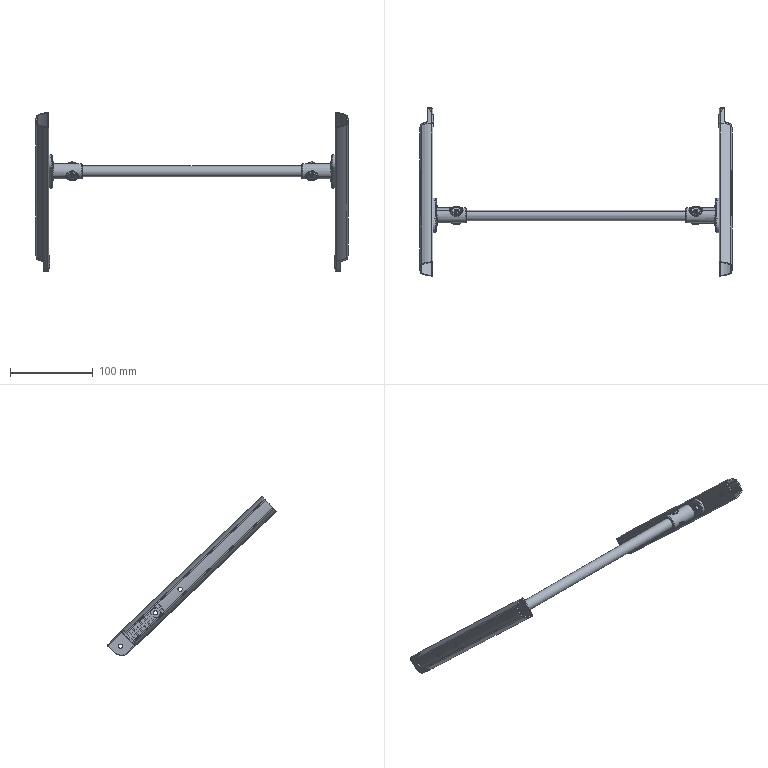Part | SolidWorks | 7 solids | 718 faces | box 377 x 203.126 x 191.613 mm | volume 96779 mm3 | plane 322 | cylinder 246 | spline 144 | cone 6 | commonest cylinder face diameters 5.2 x40 3.137 x36 0.98 x23 10.98 x10 2.941 x8 5.098 x8